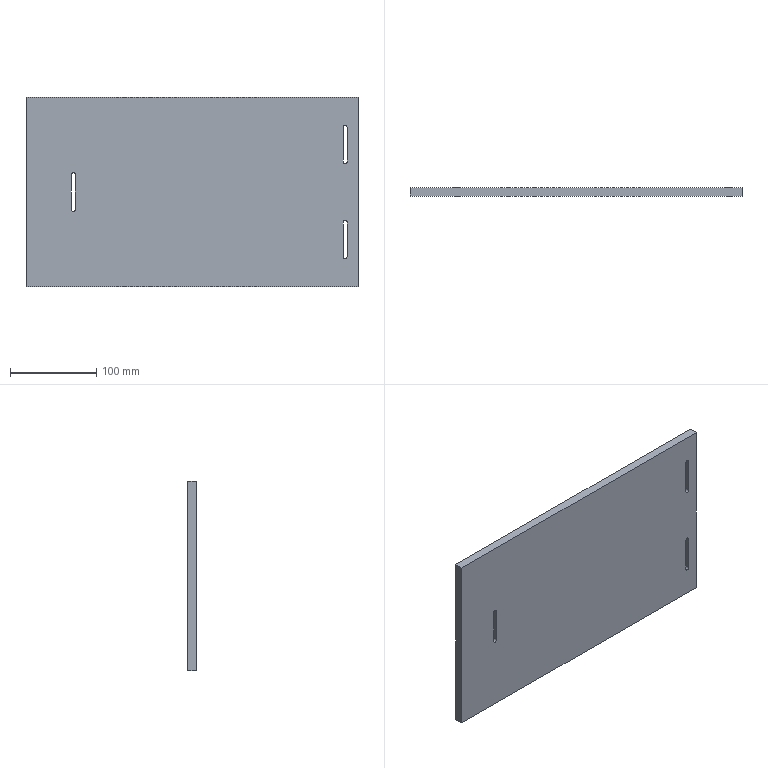Part | STEP file | Mounting plate | 1 solid | 39 faces | box 385 x 10 x 220 mm | volume 838731 mm3 | plane 21 | cylinder 18 | commonest cylinder face diameters 4.5 x9 8 x9